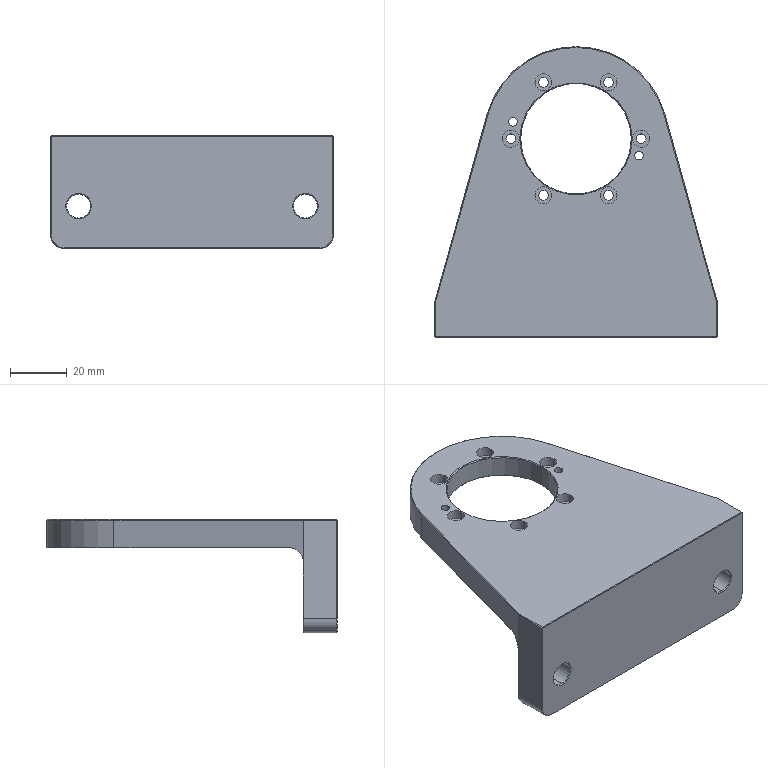NC program | NX | posted with a generic post | part box 100 x 102.5 x 40 mm
Lines 1 to 1021 of 2296:
N10 G17 G21 G94 G90
(ZLEVEL_PROFILE , TOOL : D10)
N12 T15 M6
N14 G54
N16 G17 G0 G90 X48.077 Y-38.327 B0. C0. S9500 M3
N18 G43 Z30. H15
N20 Z6.5
N22 G94 G1 X55.055 Y-13.416 Z5.144 F1000.
N24 X55.207 Y-12.875 Z5.115
N26 X55.25 Y-12.562 Z5.098
N28 Y0.262 Z4.426
N30 X54.878 Y1.721 Z4.347
N32 X54.11 Y3.015 Z4.268
N34 X53.015 Y4.11 Z4.187
N36 X51.721 Y4.878 Z4.108
N38 X50.262 Y5.25 Z4.029
N40 X49.7 Z4.
N42 X-49.7 F2000.
N44 G3 X-53.412 Y3.712 R5.25
N46 G1 X-53.712 Y3.412
N48 G3 X-55.25 Y-0.3 R5.25
N50 G1 Y-12.
N52 G3 X-55.055 Y-13.416 R5.25
N54 G1 X-36.35 Y-80.184
N56 G3 X36.35 Y-80.184 R37.75
N58 G1 X55.055 Y-13.416
N60 G3 X55.25 Y-12. R5.25
N62 G1 Y-0.3
N64 G3 X53.712 Y3.412 R5.25
N66 G1 X53.412 Y3.712
N68 G3 X49.7 Y5.25 R5.25
N70 G1 X49.313 Z3.993
N72 X-7.203 Z3.007
N74 X-7.59 Z3.
N76 X-49.7
N78 G3 X-53.412 Y3.712 R5.25
N80 G1 X-53.712 Y3.412
N82 G3 X-55.25 Y-0.3 R5.25
N84 G1 Y-12.
N86 G3 X-55.055 Y-13.416 R5.25
N88 G1 X-36.35 Y-80.184
N90 G3 X36.35 Y-80.184 R37.75
N92 G1 X55.055 Y-13.416
N94 G3 X55.25 Y-12. R5.25
N96 G1 Y-0.3
N98 G3 X53.712 Y3.412 R5.25
N100 G1 X53.412 Y3.712
N102 G3 X49.7 Y5.25 R5.25
N104 G1 X49.313 Z2.993
N106 X-7.203 Z2.007
N108 X-7.59 Z2.
N110 X-49.7
N112 G3 X-53.412 Y3.712 R5.25
N114 G1 X-53.712 Y3.412
N116 G3 X-55.25 Y-0.3 R5.25
N118 G1 Y-12.
N120 G3 X-55.055 Y-13.416 R5.25
N122 G1 X-36.35 Y-80.184
N124 G3 X36.35 Y-80.184 R37.75
N126 G1 X55.055 Y-13.416
N128 G3 X55.25 Y-12. R5.25
N130 G1 Y-0.3
N132 G3 X53.712 Y3.412 R5.25
N134 G1 X53.412 Y3.712
N136 G3 X49.7 Y5.25 R5.25
N138 G1 X49.313 Z1.993
N140 X-7.203 Z1.007
N142 X-7.59 Z1.
N144 X-49.7
N146 G3 X-53.412 Y3.712 R5.25
N148 G1 X-53.712 Y3.412
N150 G3 X-55.25 Y-0.3 R5.25
N152 G1 Y-12.
N154 G3 X-55.055 Y-13.416 R5.25
N156 G1 X-36.35 Y-80.184
N158 G3 X36.35 Y-80.184 R37.75
N160 G1 X55.055 Y-13.416
N162 G3 X55.25 Y-12. R5.25
N164 G1 Y-0.3
N166 G3 X53.712 Y3.412 R5.25
N168 G1 X53.412 Y3.712
N170 G3 X49.7 Y5.25 R5.25
N172 G1 X49.313 Z0.993
N174 X-7.203 Z0.007
N176 X-7.59 Z0.
N178 X-49.7
N180 G3 X-53.412 Y3.712 R5.25
N182 G1 X-53.712 Y3.412
N184 G3 X-55.25 Y-0.3 R5.25
N186 G1 Y-12.
N188 G3 X-55.055 Y-13.416 R5.25
N190 G1 X-36.35 Y-80.184
N192 G3 X36.35 Y-80.184 R37.75
N194 G1 X55.055 Y-13.416
N196 G3 X55.25 Y-12. R5.25
N198 G1 Y-0.3
N200 G3 X53.712 Y3.412 R5.25
N202 G1 X53.412 Y3.712
N204 G3 X49.7 Y5.25 R5.25
N206 G1 X49.313 Z-0.007
N208 X-7.203 Z-0.993
N210 X-7.59 Z-1.
N212 X-49.7
N214 G3 X-53.412 Y3.712 R5.25
N216 G1 X-53.712 Y3.412
N218 G3 X-55.25 Y-0.3 R5.25
N220 G1 Y-12.
N222 G3 X-55.055 Y-13.416 R5.25
N224 G1 X-36.35 Y-80.184
N226 G3 X36.35 Y-80.184 R37.75
N228 G1 X55.055 Y-13.416
N230 G3 X55.25 Y-12. R5.25
N232 G1 Y-0.3
N234 G3 X53.712 Y3.412 R5.25
N236 G1 X53.412 Y3.712
N238 G3 X49.7 Y5.25 R5.25
N240 G1 X-7.59
N242 Z0.5
N244 G0 Z30.
N246 M5
(FLOOR_WALL_COPY_COPY , TOOL : D80)
N248 T19 M6
N250 G54
N252 G17 G0 G90 X-95. Y-0.003 B0. C0. S6500 M3
N254 G43 Z30. H19
N256 Z7.
N258 G94 G1 Z4. F1500.
N260 X-90.
N262 X90.
N264 Y-35.251
N266 X-90.
N268 Y-70.5
N270 X90.
N272 X95.
N274 Z7.
N276 G0 Z30.
N278 X-95. Y-0.003
N280 Z6.
N282 G1 Z3.
N284 X-90.
N286 X90.
N288 Y-35.251
N290 X-90.
N292 Y-70.5
N294 X90.
N296 X95.
N298 Z6.
N300 G0 Z30.
N302 X-95. Y-0.003
N304 Z5.
N306 G1 Z2.
N308 X-90.
N310 X90.
N312 Y-35.251
N314 X-90.
N316 Y-70.5
N318 X90.
N320 X95.
N322 Z5.
N324 G0 Z30.
N326 X-95. Y-0.003
N328 Z4.
N330 G1 Z1.
N332 X-90.
N334 X90.
N336 Y-35.251
N338 X-90.
N340 Y-70.5
N342 X90.
N344 X95.
N346 Z4.
N348 G0 Z30.
N350 X-95. Y-0.003
N352 Z3.
N354 G1 Z0.
N356 X-90.
N358 X90.
N360 Y-35.251
N362 X-90.
N364 Y-70.5
N366 X90.
N368 X95.
N370 Z3.
N372 G0 Z30.
N374 M5
(FLOOR_WALL , TOOL : D10)
N376 T15 M6
N378 G54
N380 G17 G0 G90 X-3.237 Y-115.385 B0. C0. S9500 M3
N382 G43 Z30. H15
N384 Z-26.85
N386 G94 G1 Z-29.85 F1000.
N388 X-3.031 Y-112.5
N390 X-0.031
N392 X0.031 F2000.
N394 G3 X6.485 Y-112.002 R42.5
N396 G1 X-6.485
N398 G2 X-9.144 Y-111.505 R42.5
N400 G1 X9.144
N402 G3 X11.166 Y-111.007 R42.5
N404 G1 X-11.166
N406 G2 X-12.854 Y-110.509 R42.5
N408 G1 X12.854
N410 G3 X14.329 Y-110.012 R42.5
N412 G1 X-14.329
N414 G2 X-15.649 Y-109.514 R42.5
N416 G1 X15.649
N418 G3 X16.851 Y-109.017 R42.5
N420 G1 X-16.851
N422 G2 X-17.96 Y-108.519 R42.5
N424 G1 X17.96
N426 G3 X18.99 Y-108.021 R42.5
N428 G1 X-18.99
N430 G2 X-19.956 Y-107.524 R42.5
N432 G1 X19.956
N434 G3 X20.865 Y-107.026 R42.5
N436 G1 X-20.865
N438 G2 X-21.724 Y-106.528 R42.5
N440 G1 X21.724
N442 G3 X22.54 Y-106.031 R42.5
N444 G1 X-22.54
N446 G2 X-23.316 Y-105.533 R42.5
N448 G1 X23.316
N450 G3 X24.058 Y-105.035 R42.5
N452 G1 X-24.058
N454 G2 X-24.767 Y-104.538 R42.5
N456 G1 X24.767
N458 G3 X25.446 Y-104.04 R42.5
N460 G1 X-25.446
N462 G2 X-26.099 Y-103.542 R42.5
N464 G1 X26.099
N466 G3 X26.726 Y-103.045 R42.5
N468 G1 X-26.726
N470 G2 X-27.33 Y-102.547 R42.5
N472 G1 X27.33
N474 G3 X27.912 Y-102.05 R42.5
N476 G1 X-27.912
N478 G2 X-28.473 Y-101.552 R42.5
N480 G1 X28.473
N482 G3 X29.015 Y-101.054 R42.5
N484 G1 X-29.015
N486 G2 X-29.539 Y-100.557 R42.5
N488 G1 X29.539
N490 G3 X30.045 Y-100.059 R42.5
N492 G1 X-30.045
N494 G2 X-30.535 Y-99.561 R42.5
N496 G1 X30.535
N498 G3 X31.009 Y-99.064 R42.5
N500 G1 X-31.009
N502 G2 X-31.468 Y-98.566 R42.5
N504 G1 X31.468
N506 G3 X31.913 Y-98.068 R42.5
N508 G1 X-31.913
N510 G2 X-32.343 Y-97.571 R42.5
N512 G1 X32.343
N514 G3 X32.761 Y-97.073 R42.5
N516 G1 X-32.761
N518 G2 X-33.166 Y-96.576 R42.5
N520 G1 X33.166
N522 G3 X33.559 Y-96.078 R42.5
N524 G1 X-33.559
N526 G2 X-33.94 Y-95.58 R42.5
N528 G1 X33.94
N530 G3 X34.309 Y-95.083 R42.5
N532 G1 X-34.309
N534 G2 X-34.667 Y-94.585 R42.5
N536 G1 X34.667
N538 G3 X35.015 Y-94.087 R42.5
N540 G1 X-35.015
N542 G2 X-35.352 Y-93.59 R42.5
N544 G1 X35.352
N546 G3 X35.679 Y-93.092 R42.5
N548 G1 X-35.679
N550 G2 X-35.996 Y-92.594 R42.5
N552 G1 X35.996
N554 G3 X36.304 Y-92.097 R42.5
N556 G1 X-36.304
N558 G2 X-36.602 Y-91.599 R42.5
N560 G1 X36.602
N562 G3 X36.891 Y-91.102 R42.5
N564 G1 X-36.891
N566 G2 X-37.172 Y-90.604 R42.5
N568 G1 X37.172
N570 G3 X37.443 Y-90.106 R42.5
N572 G1 X-37.443
N574 G2 X-37.706 Y-89.609 R42.5
N576 G1 X37.706
N578 G3 X37.961 Y-89.111 R42.5
N580 G1 X-37.961
N582 G2 X-38.207 Y-88.613 R42.5
N584 G1 X38.207
N586 G3 X38.446 Y-88.116 R42.5
N588 G1 X-38.446
N590 G2 X-38.676 Y-87.618 R42.5
N592 G1 X38.676
N594 G3 X38.899 Y-87.12 R42.5
N596 G1 X-38.899
N598 G2 X-39.114 Y-86.623 R42.5
N600 G1 X39.114
N602 G3 X39.322 Y-86.125 R42.5
N604 G1 X-39.322
N606 G2 X-39.523 Y-85.628 R42.5
N608 G1 X39.523
N610 G3 X39.716 Y-85.13 R42.5
N612 G1 X-39.716
N614 G2 X-39.902 Y-84.632 R42.5
N616 G1 X39.902
N618 G3 X40.081 Y-84.135 R42.5
N620 G1 X-40.081
N622 G2 X-40.253 Y-83.637 R42.5
N624 G1 X40.253
N626 G3 X40.418 Y-83.139 R42.5
N628 G1 X-40.418
N630 G2 X-40.576 Y-82.642 R42.5
N632 G1 X40.576
N634 G3 X40.728 Y-82.144 R42.5
N636 G1 X-40.728
N638 G2 X-40.873 Y-81.646 R42.5
N640 G1 X40.873
N642 X40.924 Y-81.465
N644 X41.013 Y-81.149
N646 X-41.013
N648 X-41.152 Y-80.651
N650 X41.152
N652 X41.292 Y-80.153
N654 X-41.292
N656 X-41.431 Y-79.656
N658 X41.431
N660 X41.571 Y-79.158
N662 X-41.571
N664 X-41.71 Y-78.661
N666 X41.71
N668 X41.849 Y-78.163
N670 X-41.849
N672 X-41.989 Y-77.665
N674 X41.989
N676 X42.128 Y-77.168
N678 X-42.128
N680 X-42.268 Y-76.67
N682 X42.268
N684 X42.407 Y-76.172
N686 X-42.407
N688 X-42.547 Y-75.675
N690 X42.547
N692 X42.686 Y-75.177
N694 X-42.686
N696 X-42.825 Y-74.679
N698 X42.825
N700 X42.965 Y-74.182
N702 X-42.965
N704 X-43.104 Y-73.684
N706 X43.104
N708 X43.244 Y-73.187
N710 X-43.244
N712 X-43.383 Y-72.689
N714 X43.383
N716 X43.522 Y-72.191
N718 X-43.522
N720 X-43.662 Y-71.694
N722 X43.662
N724 X43.801 Y-71.196
N726 X-43.801
N728 X-43.941 Y-70.698
N730 X43.941
N732 X44.08 Y-70.201
N734 X-44.08
N736 X-44.219 Y-69.703
N738 X44.219
N740 X44.359 Y-69.205
N742 X-44.359
N744 X-44.498 Y-68.708
N746 X44.498
N748 X44.638 Y-68.21
N750 X-44.638
N752 X-44.777 Y-67.713
N754 X44.777
N756 X44.917 Y-67.215
N758 X-44.917
N760 X-45.056 Y-66.717
N762 X45.056
N764 X45.195 Y-66.22
N766 X-45.195
N768 X-45.335 Y-65.722
N770 X45.335
N772 X45.474 Y-65.224
N774 X-45.474
N776 X-45.614 Y-64.727
N778 X45.614
N780 X45.753 Y-64.229
N782 X-45.753
N784 X-45.892 Y-63.731
N786 X45.892
N788 X46.032 Y-63.234
N790 X-46.032
N792 X-46.171 Y-62.736
N794 X46.171
N796 X46.311 Y-62.238
N798 X-46.311
N800 X-46.45 Y-61.741
N802 X46.45
N804 X46.59 Y-61.243
N806 X-46.59
N808 X-46.729 Y-60.746
N810 X46.729
N812 X46.868 Y-60.248
N814 X-46.868
N816 X-47.008 Y-59.75
N818 X47.008
N820 X47.147 Y-59.253
N822 X-47.147
N824 X-47.287 Y-58.755
N826 X47.287
N828 X47.426 Y-58.257
N830 X-47.426
N832 X-47.565 Y-57.76
N834 X47.565
N836 X47.705 Y-57.262
N838 X-47.705
N840 X-47.844 Y-56.764
N842 X47.844
N844 X47.984 Y-56.267
N846 X-47.984
N848 X-48.123 Y-55.769
N850 X48.123
N852 X48.262 Y-55.272
N854 X-48.262
N856 X-48.402 Y-54.774
N858 X48.402
N860 X48.541 Y-54.276
N862 X-48.541
N864 X-48.681 Y-53.779
N866 X48.681
N868 X48.82 Y-53.281
N870 X-48.82
N872 X-48.96 Y-52.783
N874 X48.96
N876 X49.099 Y-52.286
N878 X-49.099
N880 X-49.238 Y-51.788
N882 X49.238
N884 X49.378 Y-51.29
N886 X-49.378
N888 X-49.517 Y-50.793
N890 X49.517
N892 X49.657 Y-50.295
N894 X-49.657
N896 X-49.796 Y-49.798
N898 X49.796
N900 X49.935 Y-49.3
N902 X-49.935
N904 X-50.075 Y-48.802
N906 X50.075
N908 X50.214 Y-48.305
N910 X-50.214
N912 X-50.354 Y-47.807
N914 X50.354
N916 X50.493 Y-47.309
N918 X-50.493
N920 X-50.633 Y-46.812
N922 X50.633
N924 X50.772 Y-46.314
N926 X-50.772
N928 X-50.911 Y-45.816
N930 X50.911
N932 X51.051 Y-45.319
N934 X-51.051
N936 X-51.19 Y-44.821
N938 X51.19
N940 X51.33 Y-44.324
N942 X-51.33
N944 X-51.469 Y-43.826
N946 X51.469
N948 X51.608 Y-43.328
N950 X-51.608
N952 X-51.748 Y-42.831
N954 X51.748
N956 X51.887 Y-42.333
N958 X-51.887
N960 X-52.027 Y-41.835
N962 X52.027
N964 X52.166 Y-41.338
N966 X-52.166
N968 X-52.305 Y-40.84
N970 X52.305
N972 X52.445 Y-40.342
N974 X-52.445
N976 X-52.584 Y-39.845
N978 X52.584
N980 X52.724 Y-39.347
N982 X-52.724
N984 X-52.863 Y-38.849
N986 X52.863
N988 X53.003 Y-38.352
N990 X-53.003
N992 X-53.142 Y-37.854
N994 X53.142
N996 X53.281 Y-37.357
N998 X-53.281
N1000 X-53.421 Y-36.859
N1002 X53.421
N1004 X53.56 Y-36.361
N1006 X-53.56
N1008 X-53.7 Y-35.864
N1010 X53.7
N1012 X53.839 Y-35.366
N1014 X-53.839
N1016 X-53.978 Y-34.868
N1018 X53.978
N1020 X54.118 Y-34.371
N1022 X-54.118
N1024 X-54.257 Y-33.873
N1026 X54.257
N1028 X54.397 Y-33.375
N1030 X-54.397
N1032 X-54.536 Y-32.878
N1034 X54.536
N1036 X54.675 Y-32.38
N1038 X-54.675
N1040 X-54.815 Y-31.883
N1042 X54.815
N1044 X54.954 Y-31.385
N1046 X-54.954
N1048 X-55.094 Y-30.887
N1050 X55.094
N1052 X55.233 Y-30.39
N1054 X-55.233
N1056 X-55.373 Y-29.892
N1058 X55.373
N1060 X55.512 Y-29.394
N1062 X-55.512
N1064 X-55.651 Y-28.897
N1066 X55.651
N1068 X55.791 Y-28.399
N1070 X-55.791
N1072 X-55.93 Y-27.901
N1074 X55.93
N1076 X56.07 Y-27.404
N1078 X-56.07
N1080 X-56.209 Y-26.906
N1082 X56.209
N1084 X56.348 Y-26.409
N1086 X-56.348
N1088 X-56.488 Y-25.911
N1090 X56.488
N1092 X56.627 Y-25.413
N1094 X-56.627
N1096 X-56.767 Y-24.916
N1098 X56.767
N1100 X56.906 Y-24.418
N1102 X-56.906
N1104 X-57.046 Y-23.92
N1106 X57.046
N1108 X57.185 Y-23.423
N1110 X-57.185
N1112 X-57.324 Y-22.925
N1114 X57.324
N1116 X57.464 Y-22.427
N1118 X-57.464
N1120 X-57.603 Y-21.93
N1122 X57.603
N1124 X57.743 Y-21.432
N1126 X-57.743
N1128 X-57.882 Y-20.934
N1130 X57.882
N1132 X60.998
N1134 Z-26.85
N1136 G0 Z30.
(ZLEVEL_PROFILE_COPY , TOOL : D10)
N1138 X56.587 Y-18.837
N1140 Z-0.997
N1142 G1 X55.793 Y-17.551 F1000.
N1144 G3 X54.912 Y-17.077 R1.
N1146 G1 X54.331 Y-17.094 F3000.
N1148 X48.165 Y-17.095
N1150 X47.994 Y-17.1
N1152 X-49.963
N1154 X-50.06 Y-17.095
N1156 X-54.331 Y-17.094
N1158 X-54.912 Y-17.077
N1160 G3 X-55.793 Y-17.551 R1.
N1162 G1 X-56.587 Y-18.837
N1164 G0 X-56.728 Y-18.893 Z-1.993
N1166 G1 X-55.977 Y-17.593 F1000.
N1168 G2 X-55.111 Y-17.093 R1.
N1170 G1 X-50.06 Y-17.095 F3000.
N1172 X-49.963 Y-17.1
N1174 X48.994
N1176 X49.707 Y-17.094
N1178 X55.111 Y-17.093
N1180 G2 X55.977 Y-17.593 R1.
N1182 G1 X56.727 Y-18.891
N1184 G0 X56.774 Y-18.946 Z-2.99
N1186 G1 X55.993 Y-17.593 F1000.
N1188 G3 X55.127 Y-17.093 R1.
N1190 G1 X49.707 Y-17.094 F3000.
N1192 X49.576 Y-17.1
N1194 X-49.963
N1196 X-50.06 Y-17.095
N1198 X-55.127 Y-17.093
N1200 G3 X-55.993 Y-17.593 R1.
N1202 G1 X-56.775 Y-18.946
N1204 G0 X-56.804 Y-18.97 Z-3.987
N1206 G1 X-56.009 Y-17.594 F1000.
N1208 G2 X-55.143 Y-17.094 R1.
N1210 G1 X-50.06 Y-17.096 F3000.
N1212 X-49.963 Y-17.1
N1214 X49.707
N1216 X50.477 Y-17.096
N1218 X55.143 Y-17.094
N1220 G2 X56.009 Y-17.594 R1.
N1222 G1 X56.804 Y-18.97
N1224 G0 X56.825 Y-18.978 Z-4.983
N1226 G1 X56.025 Y-17.594 F1000.
N1228 G3 X55.159 Y-17.094 R1.
N1230 G1 X50.477 Y-17.096 F3000.
N1232 X49.707 Y-17.1
N1234 X-49.999
N1236 X-50.06 Y-17.096
N1238 X-55.159 Y-17.094
N1240 G3 X-56.025 Y-17.594 R1.
N1242 G1 X-56.825 Y-18.978
N1244 G0 X-56.839 Y-18.974 Z-5.98
N1246 G1 X-56.041 Y-17.594 F1000.
N1248 G2 X-55.175 Y-17.094 R1.
N1250 G1 X-50.814 Y-17.096 F3000.
N1252 X-50.758 Y-17.043
N1254 X-49.963 Y-17.1
N1256 X49.707
N1258 X50.477 Y-17.096
N1260 X55.175 Y-17.094
N1262 G2 X56.041 Y-17.594 R1.
N1264 G1 X56.839 Y-18.974
N1266 G0 X56.853 Y-18.971 Z-6.977
N1268 G1 X56.057 Y-17.594 F1000.
N1270 G3 X55.191 Y-17.094 R1.
N1272 G1 X50.477 Y-17.096 F3000.
N1274 X49.707 Y-17.1
N1276 X-50.
N1278 X-50.758 Y-17.043
N1280 X-50.814 Y-17.096
N1282 X-55.191 Y-17.094
N1284 G3 X-56.057 Y-17.594 R1.
N1286 G1 X-56.853 Y-18.971
N1288 G0 X-56.867 Y-18.967 Z-7.973
N1290 G1 X-56.073 Y-17.594 F1000.
N1292 G2 X-55.207 Y-17.094 R1.
N1294 G1 X-50.814 Y-17.096 F3000.
N1296 X-50.758 Y-17.043
N1298 X-49.963 Y-17.1
N1300 X49.707
N1302 X50.477 Y-17.096
N1304 X55.207 Y-17.094
N1306 G2 X56.073 Y-17.594 R1.
N1308 G1 X56.867 Y-18.967
N1310 G0 X56.881 Y-18.964 Z-8.97
N1312 G1 X56.089 Y-17.594 F1000.
N1314 G3 X55.223 Y-17.094 R1.
N1316 G1 X50.477 Y-17.097 F3000.
N1318 X49.707 Y-17.1
N1320 X-50.
N1322 X-50.758 Y-17.043
N1324 X-50.814 Y-17.097
N1326 X-55.223 Y-17.094
N1328 G3 X-56.089 Y-17.594 R1.
N1330 G1 X-56.881 Y-18.964
N1332 G0 X-56.895 Y-18.96 Z-9.967
N1334 G1 X-56.105 Y-17.594 F1000.
N1336 G2 X-55.239 Y-17.094 R1.
N1338 G1 X-50.814 Y-17.097 F3000.
N1340 X-50.758 Y-17.043
N1342 X-49.963 Y-17.1
N1344 X49.707
N1346 X50.477 Y-17.097
N1348 X55.239 Y-17.094
N1350 G2 X56.105 Y-17.594 R1.
N1352 G1 X56.895 Y-18.96
N1354 G0 X56.943 Y-18.95 Z-10.963
N1356 G1 X56.128 Y-17.582 F1000.
N1358 G3 X55.255 Y-17.094 R1.
N1360 G1 X55.101 Y-17.096 F3000.
N1362 X50.477 Y-17.097
N1364 X49.707 Y-17.1
N1366 X-50.
N1368 X-50.758 Y-17.043
N1370 X-50.814 Y-17.097
N1372 X-55.101 Y-17.096
N1374 X-55.255 Y-17.094
N1376 G3 X-56.128 Y-17.582 R1.
N1378 G1 X-56.943 Y-18.95
N1380 G0 X-56.958 Y-18.946 Z-11.96
N1382 G1 X-56.144 Y-17.582 F1000.
N1384 G2 X-55.271 Y-17.094 R1.
N1386 G1 X-55.101 Y-17.097 F3000.
N1388 X-50.814
N1390 X-50.758 Y-17.043
N1392 X-50. Y-17.1
N1394 X49.707
N1396 X50.477 Y-17.097
N1398 X55.101
N1400 X55.271 Y-17.094
N1402 G2 X56.144 Y-17.582 R1.
N1404 G1 X56.958 Y-18.946
N1406 G0 X56.972 Y-18.942 Z-12.957
N1408 G1 X56.16 Y-17.582 F1000.
N1410 G3 X55.287 Y-17.094 R1.
N1412 G1 X55.101 Y-17.097 F3000.
N1414 X50.477 Y-17.098
N1416 X49.707 Y-17.1
N1418 X-50. Y-17.101
N1420 X-50.758 Y-17.043
N1422 X-50.814 Y-17.098
N1424 X-55.101 Y-17.097
N1426 X-55.287 Y-17.094
N1428 G3 X-56.16 Y-17.582 R1.
N1430 G1 X-56.972 Y-18.942
N1432 G0 X-56.987 Y-18.939 Z-13.953
N1434 G1 X-56.176 Y-17.581 F1000.
N1436 G2 X-55.303 Y-17.094 R1.
N1438 G1 X-55.101 Y-17.097 F3000.
N1440 X-50.814 Y-17.098
N1442 X-50.758 Y-17.043
N1444 X-50. Y-17.101
N1446 X49.707 Y-17.1
N1448 X50.477 Y-17.098
N1450 X55.101 Y-17.097
N1452 X55.303 Y-17.094
N1454 G2 X56.176 Y-17.581 R1.
N1456 G1 X56.987 Y-18.939
N1458 G0 X57.002 Y-18.935 Z-14.95
N1460 G1 X56.193 Y-17.581 F1000.
N1462 G3 X55.319 Y-17.094 R1.
N1464 G1 X55.101 Y-17.097 F3000.
N1466 X49.707 Y-17.1
N1468 X-50. Y-17.101
N1470 X-50.758 Y-17.043
N1472 X-50.814 Y-17.098
N1474 X-55.101 Y-17.097
N1476 X-55.319 Y-17.094
N1478 G3 X-56.193 Y-17.581 R1.
N1480 G1 X-57.002 Y-18.935
N1482 G0 X-57.016 Y-18.931 Z-15.947
N1484 G1 X-56.209 Y-17.581 F1000.
N1486 G2 X-55.335 Y-17.094 R1.
N1488 G1 X-55.101 Y-17.098 F3000.
N1490 X-50.814
N1492 X-50.758 Y-17.043
N1494 X-50. Y-17.101
N1496 X49.707 Y-17.1
N1498 X55.101 Y-17.098
N1500 X55.335 Y-17.094
N1502 G2 X56.209 Y-17.581 R1.
N1504 G1 X57.016 Y-18.931
N1506 G0 X57.031 Y-18.928 Z-16.943
N1508 G1 X56.225 Y-17.581 F1000.
N1510 G3 X55.351 Y-17.094 R1.
N1512 G1 X55.101 Y-17.098 F3000.
N1514 X49.707 Y-17.1
N1516 X-50. Y-17.101
N1518 X-50.758 Y-17.043
N1520 X-50.814 Y-17.098
N1522 X-55.101
N1524 X-55.351 Y-17.094
N1526 G3 X-56.225 Y-17.581 R1.
N1528 G1 X-57.031 Y-18.928
N1530 G0 X-57.045 Y-18.924 Z-17.94
N1532 G1 X-56.241 Y-17.58 F1000.
N1534 G2 X-55.367 Y-17.094 R1.
N1536 G1 X-55.101 Y-17.098 F3000.
N1538 X-50.814 Y-17.099
N1540 X-50.758 Y-17.043
N1542 X-50. Y-17.101
N1544 X49.707 Y-17.1
N1546 X55.101 Y-17.098
N1548 X55.367 Y-17.094
N1550 G2 X56.241 Y-17.58 R1.
N1552 G1 X57.045 Y-18.924
N1554 G0 X57.06 Y-18.92 Z-18.937
N1556 G1 X56.257 Y-17.58 F1000.
N1558 G3 X55.383 Y-17.094 R1.
N1560 G1 X55.101 Y-17.098 F3000.
N1562 X49.707 Y-17.1
N1564 X-50. Y-17.101
N1566 X-50.758 Y-17.043
N1568 X-50.814 Y-17.099
N1570 X-55.101 Y-17.098
N1572 X-55.383 Y-17.094
N1574 G3 X-56.257 Y-17.58 R1.
N1576 G1 X-57.06 Y-18.92
N1578 G0 X-57.074 Y-18.917 Z-19.933
N1580 G1 X-56.273 Y-17.58 F1000.
N1582 G2 X-55.399 Y-17.094 R1.
N1584 G1 X-55.101 Y-17.099 F3000.
N1586 X-50.814
N1588 X-50.758 Y-17.043
N1590 X-50. Y-17.101
N1592 X49.707 Y-17.1
N1594 X55.101 Y-17.099
N1596 X55.399 Y-17.094
N1598 G2 X56.273 Y-17.58 R1.
N1600 G1 X57.075 Y-18.917
N1602 G0 X57.089 Y-18.913 Z-20.93
N1604 G1 X56.289 Y-17.579 F1000.
N1606 G3 X55.415 Y-17.094 R1.
N1608 G1 X55.101 Y-17.099 F3000.
N1610 X49.707 Y-17.1
N1612 X-50. Y-17.101
N1614 X-50.758 Y-17.043
N1616 X-50.814 Y-17.099
N1618 X-55.101
N1620 X-55.415 Y-17.094
N1622 G3 X-56.289 Y-17.579 R1.
N1624 G1 X-57.089 Y-18.913
N1626 G0 X-57.104 Y-18.909 Z-21.927
N1628 G1 X-56.305 Y-17.579 F1000.
N1630 G2 X-55.431 Y-17.094 R1.
N1632 G1 X-55.101 Y-17.099 F3000.
N1634 X-50.814
N1636 X-50.758 Y-17.043
N1638 X-50. Y-17.101
N1640 X49.707 Y-17.1
N1642 X55.101 Y-17.099
N1644 X55.431 Y-17.094
N1646 G2 X56.306 Y-17.579 R1.
N1648 G1 X57.104 Y-18.91
N1650 G0 X57.118 Y-18.906 Z-22.923
N1652 G1 X56.322 Y-17.579 F1000.
N1654 G3 X55.447 Y-17.094 R1.
N1656 G1 X55.101 Y-17.099 F3000.
N1658 X49.707 Y-17.1
N1660 X-50. Y-17.101
N1662 X-50.758 Y-17.043
N1664 X-50.814 Y-17.1
N1666 X-55.101 Y-17.099
N1668 X-55.447 Y-17.094
N1670 G3 X-56.322 Y-17.579 R1.
N1672 G1 X-57.118 Y-18.906
N1674 G0 X-57.133 Y-18.902 Z-23.92
N1676 G1 X-56.338 Y-17.578 F1000.
N1678 G2 X-55.463 Y-17.093 R1.
N1680 G1 X-55.101 Y-17.1 F3000.
N1682 X-50.814
N1684 X-50.758 Y-17.043
N1686 X-50. Y-17.101
N1688 X49.707 Y-17.1
N1690 X55.101
N1692 X55.463 Y-17.093
N1694 G2 X56.338 Y-17.578 R1.
N1696 G1 X57.133 Y-18.902
N1698 G0 X57.148 Y-18.899 Z-24.917
N1700 G1 X56.354 Y-17.578 F1000.
N1702 G3 X55.479 Y-17.093 R1.
N1704 G1 X55.101 Y-17.1 F3000.
N1706 X49.707
N1708 X-50. Y-17.101
N1710 X-50.758 Y-17.043
N1712 X-50.814 Y-17.1
N1714 X-55.101
N1716 X-55.479 Y-17.093
N1718 G3 X-56.354 Y-17.578 R1.
N1720 G1 X-57.148 Y-18.899
N1722 G0 X-57.087 Y-19.014 Z-25.913
N1724 G1 X-56.323 Y-17.698 F1000.
N1726 G2 X-55.456 Y-17.2 R1.
N1728 G1 X-55.101 F3000.
N1730 X-50.477 Y-17.197
N1732 X-49.975 Y-17.186
N1734 X49.975
N1736 X50.477 Y-17.197
N1738 X55.456 Y-17.2
N1740 G2 X56.322 Y-17.7 R1.
N1742 G1 X57.081 Y-19.016
N1744 G0 X57.082 Y-19.294 Z-26.91
N1746 G1 X56.275 Y-17.969 F1000.
N1748 G3 X55.397 Y-17.49 R1.
N1750 G1 X55.101 Y-17.496 F3000.
N1752 X50.477 Y-17.494
N1754 X49.889 Y-17.488
N1756 X-49.889
N1758 X-50.477 Y-17.494
N1760 X-55.101 Y-17.496
N1762 X-55.397 Y-17.49
N1764 G3 X-56.275 Y-17.969 R1.
N1766 G1 X-57.082 Y-19.294
N1768 G0 X-57.006 Y-19.858 Z-27.907
N1770 G1 X-56.151 Y-18.528 F1000.
N1772 G2 X-55.262 Y-18.07 R1.
N1774 G1 X-55.101 Y-18.078 F3000.
N1776 X-50.477 Y-18.074
N1778 X-49.726 Y-18.055
N1780 X49.726
N1782 X50.477 Y-18.074
N1784 X55.101 Y-18.078
N1786 X55.262 Y-18.07
N1788 G2 X56.151 Y-18.528 R1.
N1790 G1 X57.007 Y-19.858
N1792 G0 X56.665 Y-20.864 Z-28.903
N1794 G1 X55.914 Y-19.559 F1000.
N1796 G3 X55.049 Y-19.058 R1.
N1798 G1 X49.707 Y-19.051 F3000.
N1800 X49.445 Y-19.038
N1802 X-49.445
N1804 X-49.707 Y-19.051
N1806 X-55.049 Y-19.058
N1808 G3 X-55.914 Y-19.559 R1.
N1810 G1 X-56.667 Y-20.868
N1812 G0 X-54.49 Y-24.004 Z-29.9
N1814 G1 X-53.412 Y-22.138 F1000.
N1816 G2 X-52.979 Y-21.888 R0.5
N1818 G1 X52.979 F3000.
N1820 G2 X53.412 Y-22.138 R0.5
N1822 G1 X54.496 Y-24.015
N1824 G0 Z30.
N1826 M5
(HOLE_MILLING_COPY , TOOL : D10JING)
N1828 T14 M6
N1830 G54
N1832 G17 G0 G90 X9.659 Y-76.055 B0. C0. S9500 M3
N1834 G43 Z30. H14
N1836 Z-29.5
N1838 G94 G3 X20.6 Y-70. R7.146 F1500.
N1840 X20.6 Y-70. Z-30.5 I-20.6 J0.
N1842 X20.6 Y-70. Z-31.5 I-20.6 J0.
N1844 X-20.6 Y-70. Z-32. I-20.6 J0.
N1846 X0. Y-90.6 R20.6
N1848 X-20.6 Y-70. R-20.6
N1850 X-9.659 Y-76.055 R7.146
N1852 G0 Z30.
(ZLEVEL_PROFILE_COPY_1_COPY_COPY_1_COPY_1 , TOOL : D10JING)
N1854 X56.479 Y-18.924
N1856 Z-11.45
N1858 G1 Z-12.45 F1000.
N1860 X55.655 Y-17.497
N1862 G3 X54.789 Y-16.998 R1.
N1864 G1 X49.387 Y-17. F1200.
N1866 X-50. Y-17.001
N1868 X-50.73 Y-16.946
N1870 X-50.786 Y-16.999
N1872 X-54.789 Y-16.998
N1874 G3 X-55.655 Y-17.497 R1.
N1876 G1 X-56.478 Y-18.922
N1878 Z-11.45
N1880 G0 X56.478 Y-18.925 Z-23.9
N1882 G1 Z-24.9 F1000.
N1884 X55.655 Y-17.499
N1886 G3 X54.789 Y-16.999 R1.
N1888 G1 X49.387 Y-17. F1200.
N1890 X-50. Y-17.001
N1892 X-50.73 Y-16.946
N1894 X-50.786 Y-17.
N1896 X-54.789 Y-16.999
N1898 G3 X-55.655 Y-17.499 R1.
N1900 G1 X-56.478 Y-18.924
N1902 Z-23.9
N1904 G0 Z30.
(FLOOR_WALL_1 , TOOL : D10JING)
N1906 X24.166 Y-102.5
N1908 Z-27.
N1910 G1 Z-30. F1250.
N1912 X18.708
N1914 X-18.708
N1916 G2 X-25.495 Y-97.5 R37.5
N1918 G1 X25.495
N1920 G3 X30. Y-92.5 R37.5
N1922 G1 X-30.
N1924 G2 X-33.166 Y-87.5 R37.5
N1926 G1 X33.166
N1928 G3 X35.355 Y-82.5 R37.5
N1930 G1 X-35.355
N1932 G2 X-36.11 Y-80.116 R37.5
N1934 G1 X-36.843 Y-77.5
N1936 X36.843
N1938 X38.243 Y-72.5
N1940 X-38.243
N1942 X-39.644 Y-67.5
N1944 X39.644
N1946 X41.045 Y-62.5
N1948 X-41.045
N1950 X-42.446 Y-57.5
N1952 X42.446
N1954 X43.846 Y-52.5
N1956 X-43.846
N1958 X-45.247 Y-47.5
N1960 X45.247
N1962 X46.648 Y-42.5
N1964 X-46.648
N1966 X-48.049 Y-37.5
N1968 X48.049
N1970 X49.449 Y-32.5
N1972 X-49.449
N1974 X-50.85 Y-27.5
N1976 X50.85
N1978 X52.251 Y-22.5
N1980 X-52.251
N1982 X-55.366
N1984 Z-27.
N1986 G0 Z30.
N1988 X55.507 Y-22.
N1990 Z-27.
N1992 G1 Z-30.
N1994 X52.391
N1996 X-52.391
N1998 X-55.507
N2000 Z-27.
N2002 G0 Z30.
N2004 M5